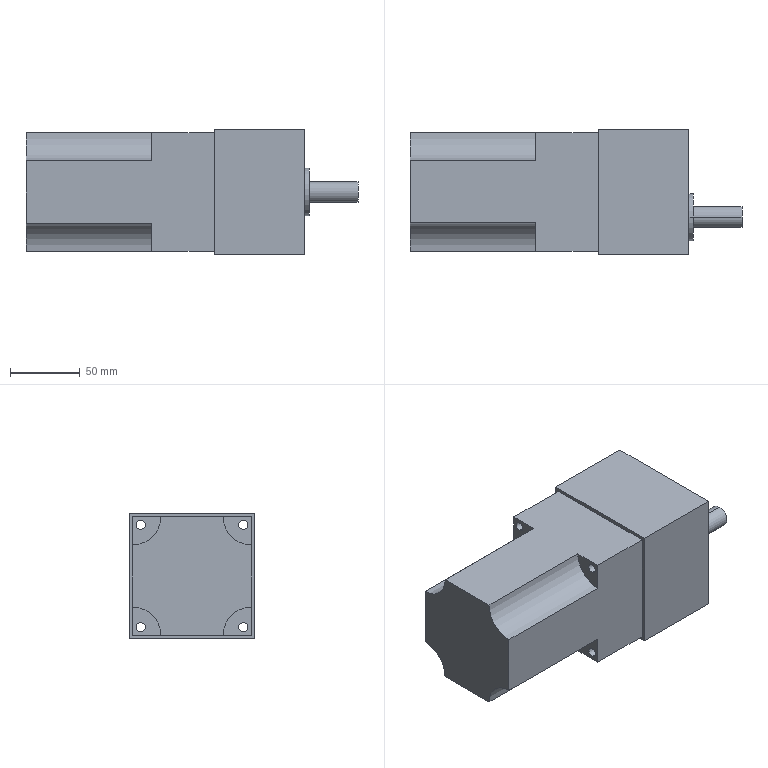Part | STEP file | PN_0060 (60W.1:15) | 1 solid | 33 faces | box 238 x 90 x 90 mm | volume 1379919 mm3 | plane 17 | cylinder 16 | commonest cylinder face diameters 6.6 x8 40.477 x4 15 x2 34 x2